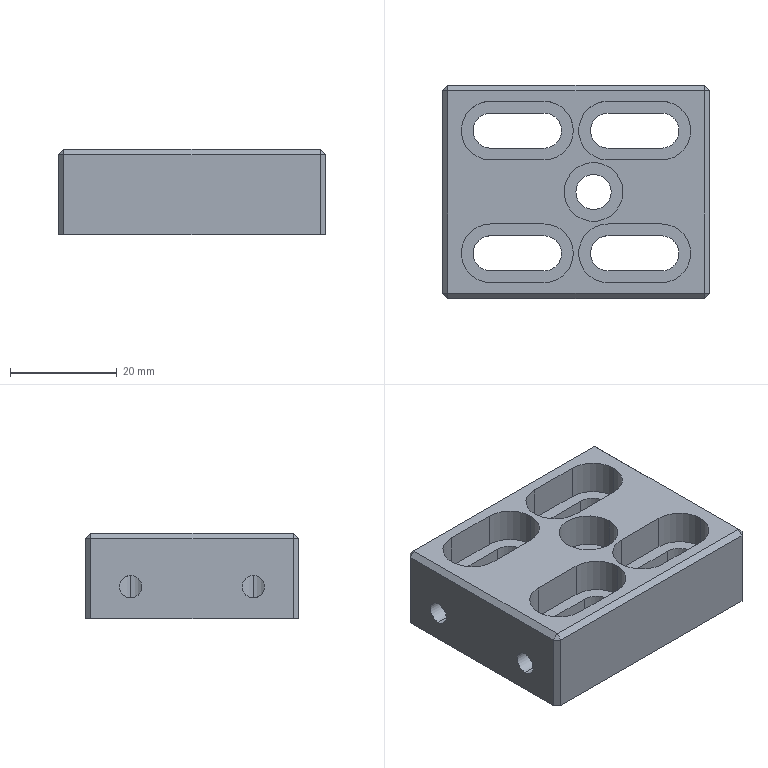Part | STEP file | Timing belt tensioner block^X moving platform_PS-3045E-LDJ | 1 solid | 74 faces | box 50 x 40 x 16 mm | volume 21271 mm3 | plane 40 | cylinder 34 | commonest cylinder face diameters 11 x16 6.6 x14 4.2 x4